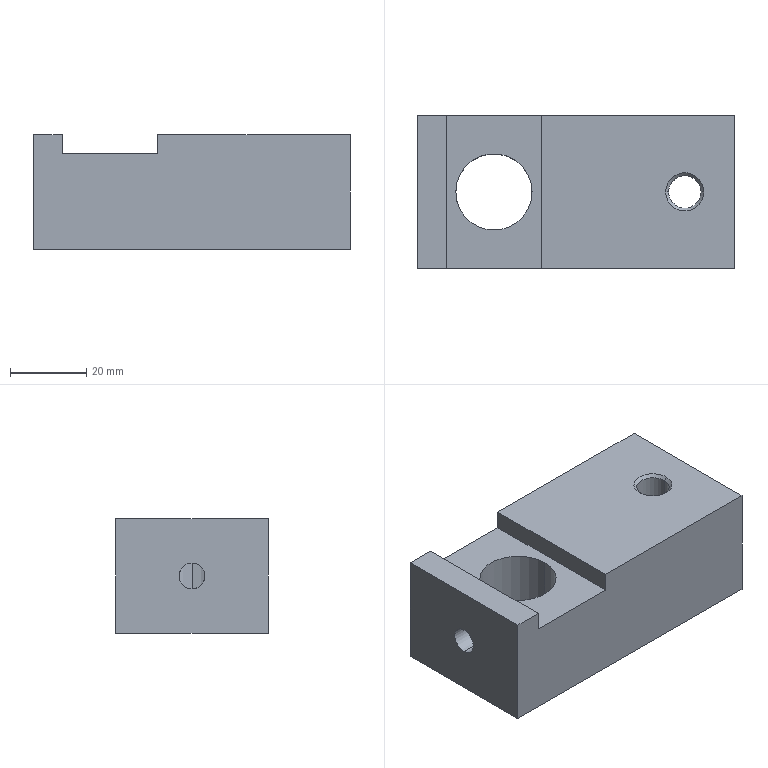Part | STEP file | BCC3 H16_12 | 1 solid | 22 faces | box 83 x 40 x 30 mm | volume 84627 mm3 | plane 10 | cone 6 | cylinder 6 | commonest cylinder face diameters 6.8 x2 8.5 x2 20 x2